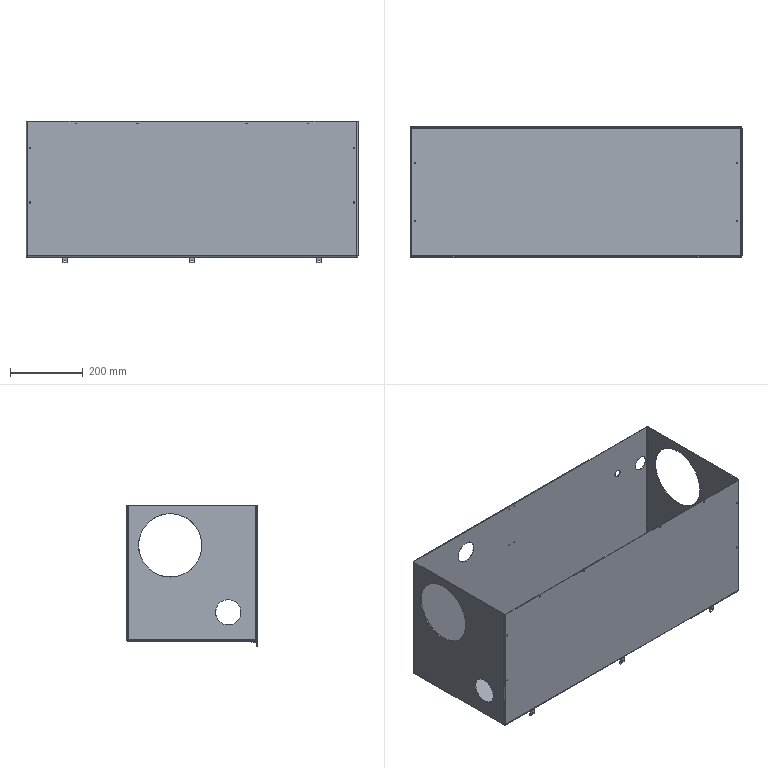Part | STEP file | 1 solid | 127 faces | box 915 x 360 x 390 mm | volume 2426206 mm3 | cylinder 64 | plane 55 | spline 8 | commonest cylinder face diameters 3.3 x24 4.5 x10 4 x8 8 x8 70 x4 175 x4